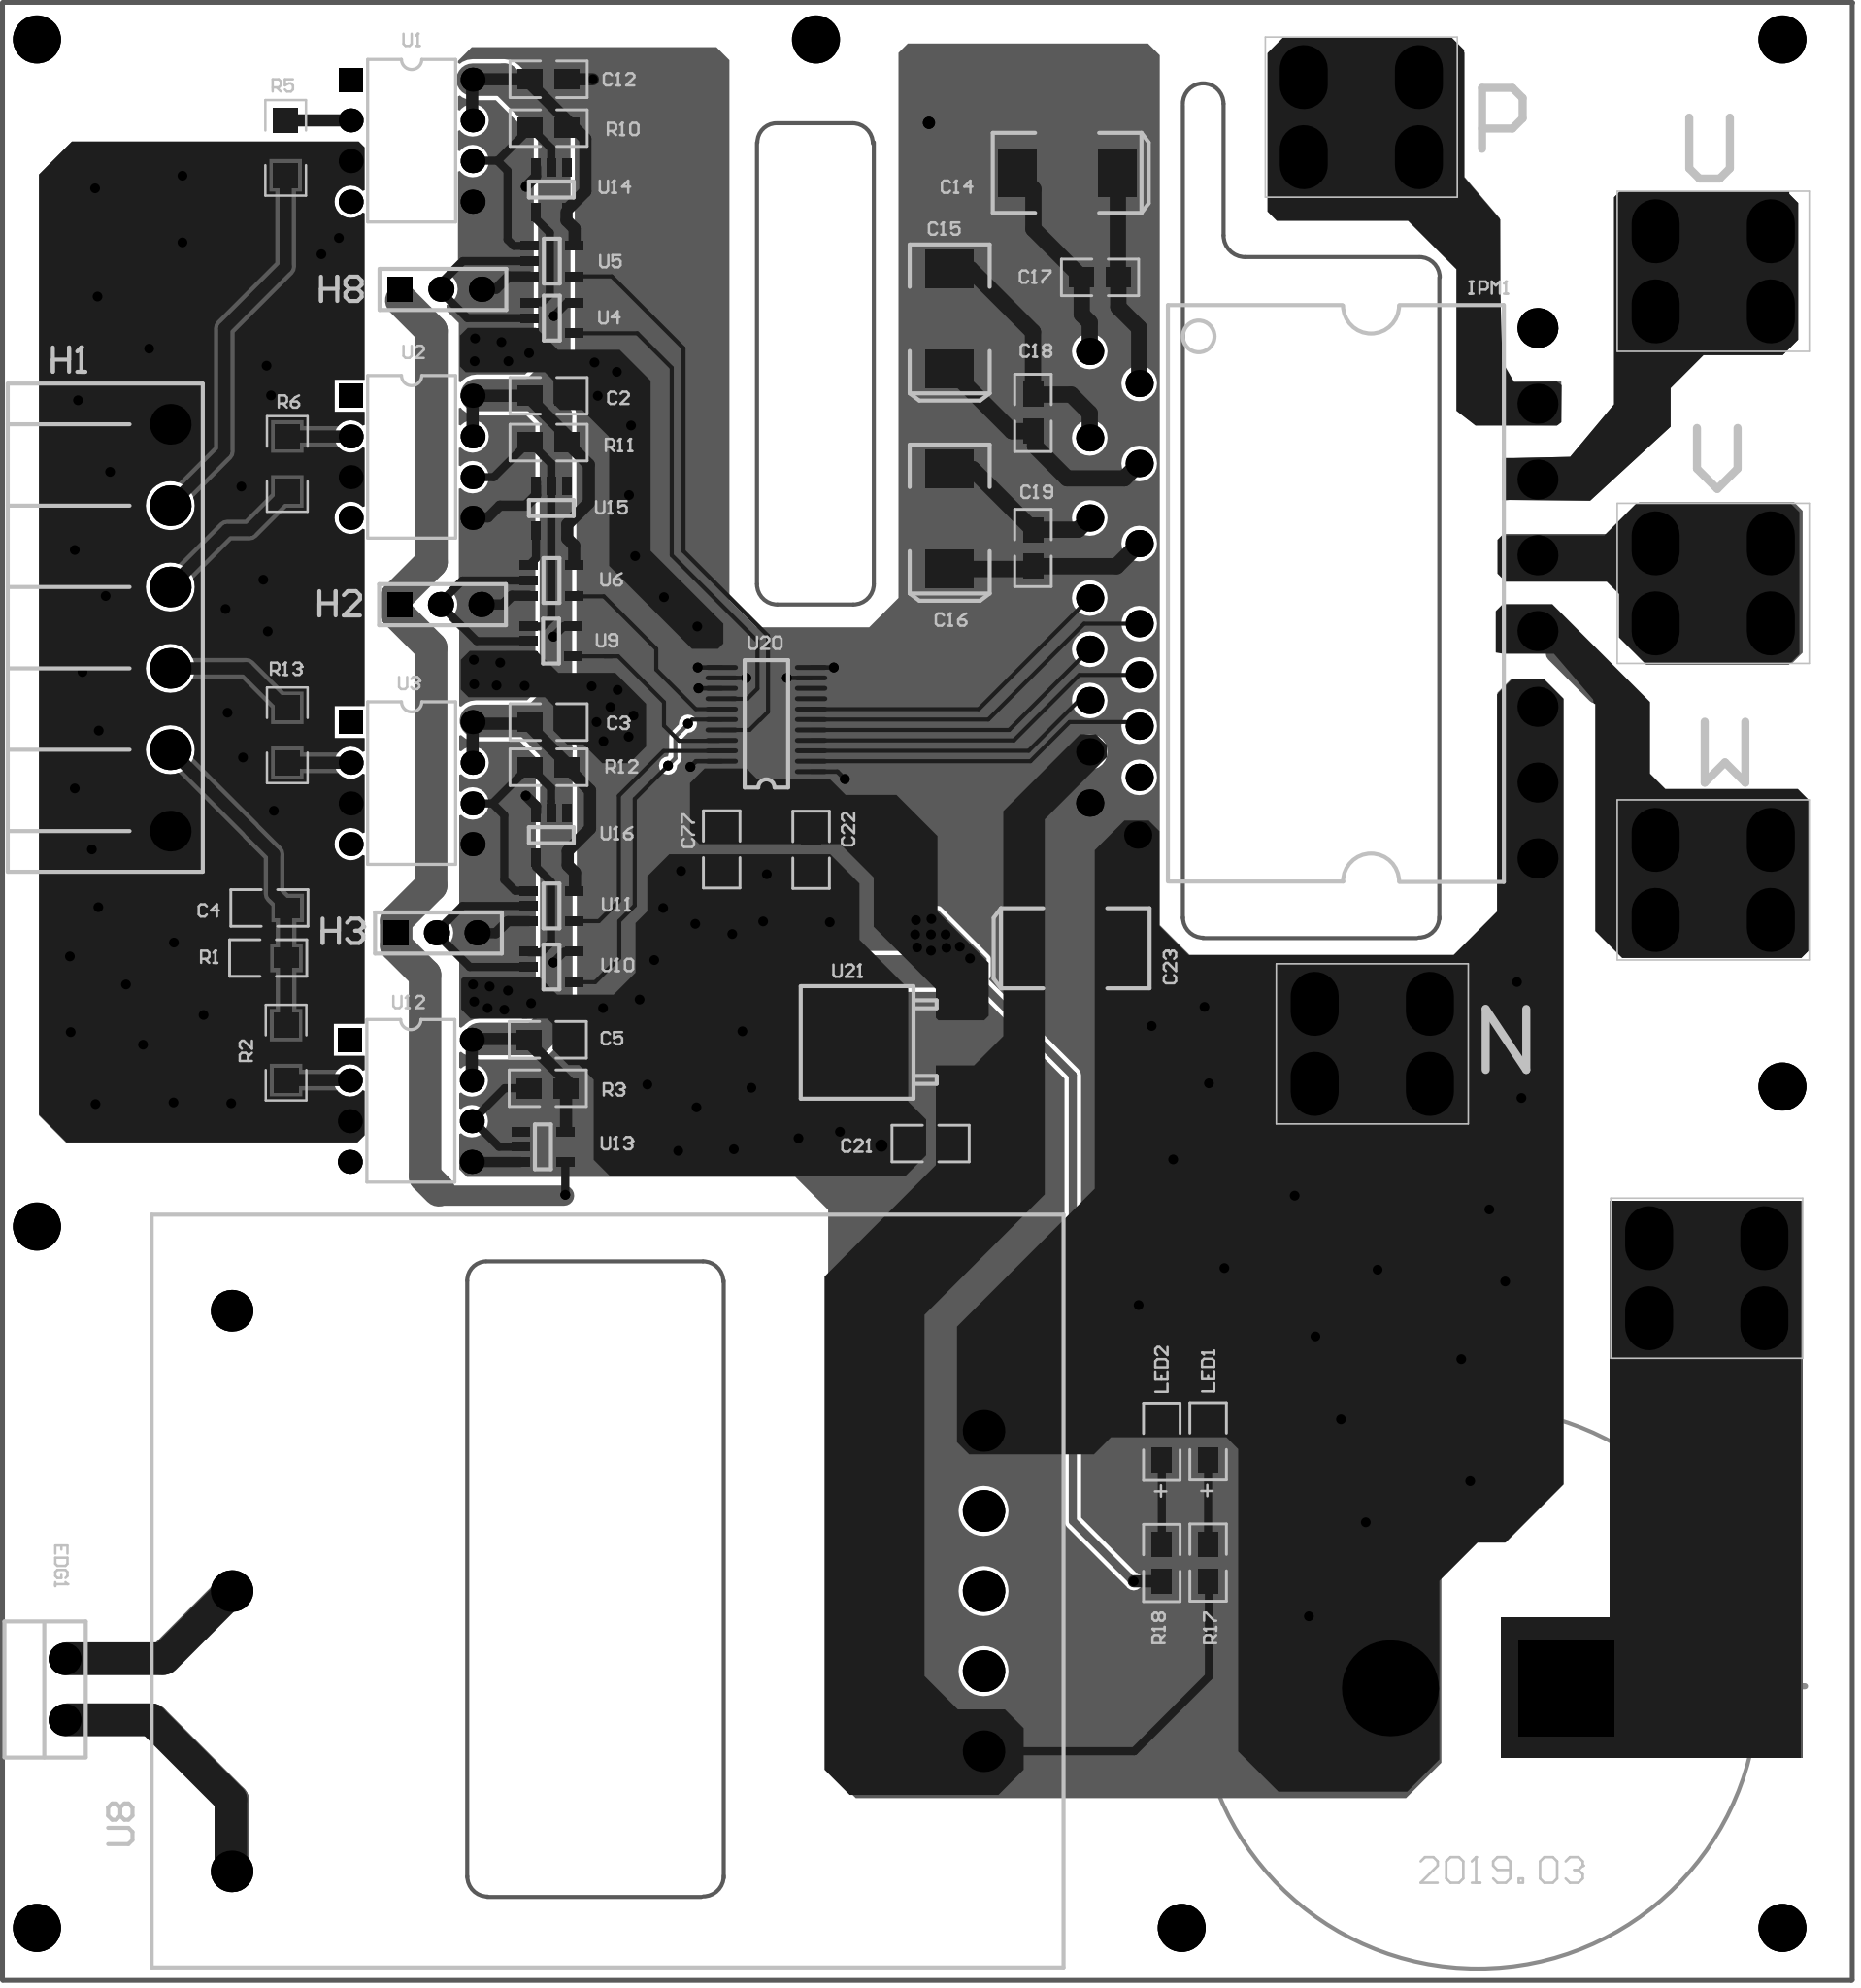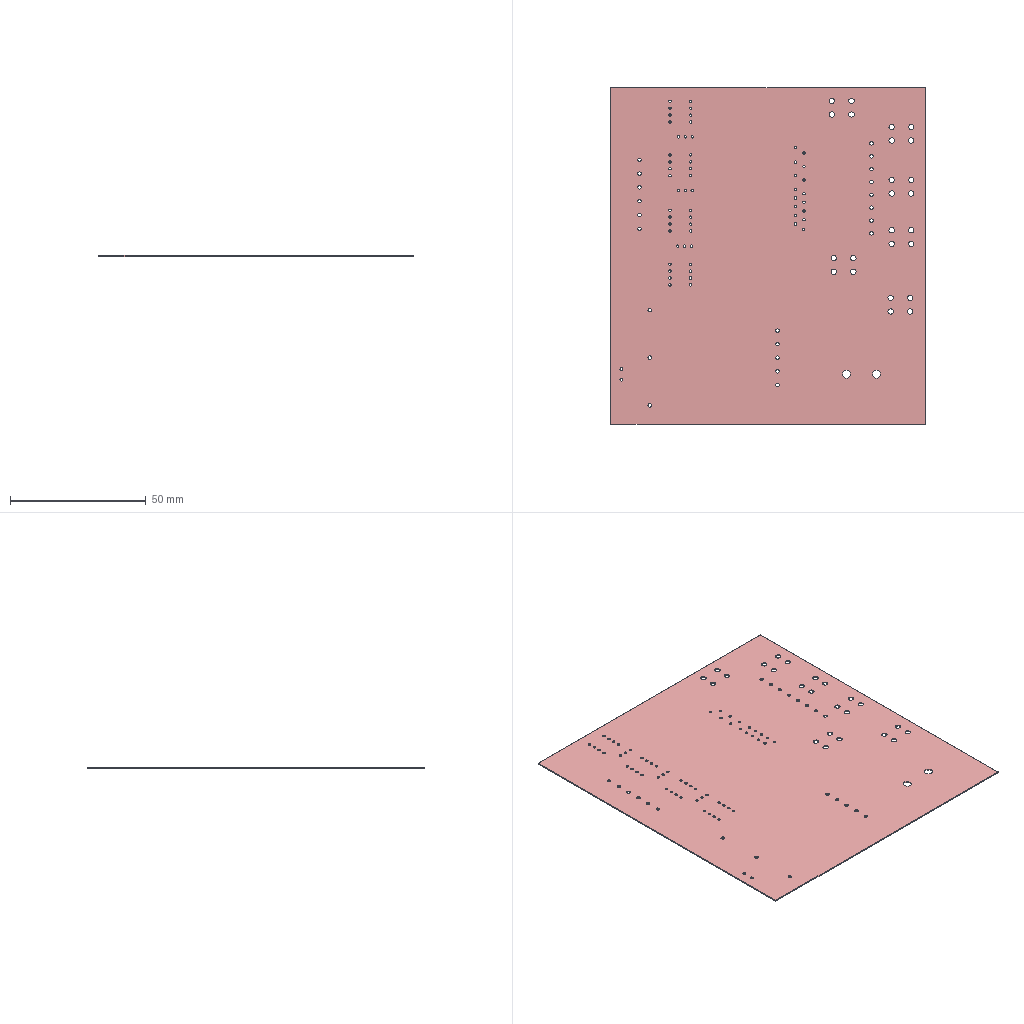Circuit board layout | Altium Designer | box 115.9 x 123.7 x 0.4 mm
Layer stack:
# Altium Designer layer stack of  (unit mm; dielectric type: 0 none, 1 core, 2 prepreg, 3 surface material)
index,name,kind,layer,copper_thickness_mm,dielectric_type,dielectric_thickness_mm,dielectric_material,dielectric_constant
0,Top Paste,other,,,,,,
1,Top Overlay,other,,,,,,
2,Top Solder,dielectric,,,3,0.0102,Solder Resist,3.5
3,Top Layer,copper,Top Layer,0.0356,,,,
4,Dielectric1,dielectric,,,0,0.32,FR-4,4.8
5,Bottom Layer,copper,Bottom Layer,0.0356,,,,
6,Bottom Solder,dielectric,,,3,0.0102,Solder Resist,3.5
7,Bottom Overlay,other,,,,,,
8,Bottom Paste,other,,,,,,
# drill layer pairs: low layer,high layer
drill_pair,Top Layer,Bottom Layer
Part placement:
Designator,Comment,Layer,Footprint,Center-X(mm),Center-Y(mm),Rotation
C22,0.01uF,TopLayer,0805,50.495,70.485,90
C1,450V,BottomLayer,ElecCap_450V,92.177,18.136,180
C19,0.1uF,TopLayer,0805,64.364,89.332,90
C15,22uF/35V,TopLayer,7343_CASE-D,59.157,103.632,270
C18,0.1uF,TopLayer,0805,64.364,97.765,90
C14,22uF/35V,TopLayer,7343_CASE-D,66.497,112.751,360
C16,22uF/35V,TopLayer,7343_CASE-D,59.157,91.135,270
C23,22uF/35V,TopLayer,7343_CASE-D,67.005,64.338,180
C17,0.1uF,TopLayer,0805,68.555,106.223,180
U21,L78M05,TopLayer,TO-252-2(DPAK),56.696,58.471,360
U20,SN74LVC8T245,TopLayer,SN74LVC8T245_TSSOP24,47.701,78.293,180
R13,500R,TopLayer,1206,17.755,77.635,90
R5,500R,TopLayer,1206,17.653,114.313,270
R6,500R,TopLayer,1206,17.755,94.577,270
U6,SN74AHC1G08,TopLayer,SOT-23-5,34.265,87.3,180
U5,SN74AHC1G08,TopLayer,SOT-23-5,34.29,107.239,180
U4,SN74AHC1G08,TopLayer,SOT-23-5,34.29,103.683,180
U3,6N137,TopLayer,DIP-8,25.527,74.651,360
U1,6N137,TopLayer,DIP-8,25.527,114.757,360
W1,PCBTerminator,TopLayer,PCBTerminator,106.883,68.605,90
IPM1,IKCM15F60GA,TopLayer,IKCM15F60GA,81.904,86.509,90
EDG1,EDG 2p,TopLayer,EDGCon_2p_3.81mm,3.835,18.059,270
N1,PCBTerminator,TopLayer,PCBTerminator,85.573,58.369,90
P1,PCBTerminator,TopLayer,PCBTerminator,84.887,116.23,90
U7,PCBTerminator,TopLayer,PCBTerminator,106.883,106.604,90
V1,PCBTerminator,TopLayer,PCBTerminator,106.883,87.122,90
C21,0.33uF,TopLayer,0805,57.963,52.146,360
U2,6N137,TopLayer,DIP-8,25.527,95.021,360
R10,10k,TopLayer,0805,34.087,115.545,360
H8,Header3,TopLayer,PinHeader3_2.54mm,27.356,105.486,360
LED1,LED,TopLayer,0805_LED,75.311,33.553,90
LED2,LED,TopLayer,0805_LED,72.415,33.528,90
R17,10k,TopLayer,0805,75.311,25.984,270
R18,3.3k,TopLayer,0805,72.415,25.959,270
U8,YAS5-15-W,TopLayer,YAS5,37.775,24.207,180
C77,0.1uF,TopLayer,0805,44.907,70.51,270
P2,PCBTerminator,TopLayer,PCBTerminator,106.477,43.739,90
U9,SN74AHC1G08,TopLayer,SOT-23-5,34.239,83.515,180
U10,SN74AHC1G08,TopLayer,SOT-23-5,34.265,63.17,180
U11,SN74AHC1G08,TopLayer,SOT-23-5,34.265,66.98,180
H1,Header6,TopLayer,EDGCon_6P_5.08mm,10.439,84.353,270
C4,30pF,TopLayer,0805,16.637,66.853,360
C5,0.1uF,TopLayer,0805,34.036,58.623,180
H2,Header3,TopLayer,PinHeader3_2.54mm,27.33,85.801,360
H3,Header3,TopLayer,PinHeader3_2.54mm,27.076,65.303,360
R1,10k,TopLayer,0805,16.561,63.729,360
R2,500R,TopLayer,1206,17.678,57.823,90
R3,10k,TopLayer,0805,34.036,55.601,360
U12,6N137,TopLayer,DIP-8,25.476,54.813,360
U13,SN74AHC1G04,TopLayer,SOT-23-5,33.731,51.943,180
C2,0.1uF,TopLayer,0805,34.087,98.831,180
C3,0.1uF,TopLayer,0805,34.087,78.461,180
C12,0.1uF,TopLayer,0805,34.087,118.593,180
R11,10k,TopLayer,0805,34.087,95.91,360
R12,10k,TopLayer,0805,34.087,75.641,360
U14,SN74AHC1G04,TopLayer,SOT-23-5,34.256,111.709,90
U15,SN74AHC1G04,TopLayer,SOT-23-5,34.256,91.821,90
U16,SN74AHC1G04,TopLayer,SOT-23-5,34.256,71.399,90
Pad and via stacks:
# Altium Designer via and pad stacks of  (unit mm). Each distinct definition once, with the count of objects using it.
# via: kind,start_layer,end_layer,hole_mm,diameter_mm,mode(0 simple;1 top-mid-bottom;2 full stack),diameter_per_layer,count,example_net
# pad: kind,layer,hole_mm,hole_type(0 round;1 square;2 slot),plating,top_size,top_shape(1 round;2 rect;3 octagon;9 rounded rect),mid_size,bottom_size,mode,footprint,size_per_layer,count,example
pad,Top Layer,0,0,plated,2.4x3,2,2.4x3,2.4x3,0,7343_CASE-D,,8,C23.1
pad,Top Layer,0,0,plated,1.524x1.27,2,1.524x1.27,1.524x1.27,0,0805,,36,C19.2
pad,Top Layer,0,0,plated,1.524x1.27,2,1.524x1.27,1.524x1.27,0,0805_LED,,4,LED2.K
pad,Top Layer,0,0,plated,1.524x1.524,2,1.524x1.524,1.524x1.524,0,1206,,8,R6.2
pad,Top Layer,0,0,plated,1.5x2.8,2,1.5x2.8,1.5x2.8,0,TO-252-2(DPAK),,2,U21.2
pad,Top Layer,0,0,plated,6.3x6.3,2,6.3x6.3,6.3x6.3,0,TO-252-2(DPAK),,1,U21.1
pad,Top Layer,0,0,plated,2.032x0.3048,1,2.032x0.3048,2.032x0.3048,0,SN74LVC8T245_TSSOP24,,23,U20.14
pad,Top Layer,0,0,plated,2.032x0.3048,2,2.032x0.3048,2.032x0.3048,0,SN74LVC8T245_TSSOP24,,1,U20.1
pad,Top Layer,0,0,plated,0.6x1.1,2,0.6x1.1,0.6x1.1,0,SOT-23-5,,50,U11.1
pad,Multi-Layer,0.8636,0,plated,1.575x1.575,1,1.575x1.575,1.575x1.575,0,PinHeader3_2.54mm,,6,H8.2
pad,Multi-Layer,0.8636,0,plated,1.575x1.575,2,1.575x1.575,1.575x1.575,0,PinHeader3_2.54mm,,3,H8.1
pad,Multi-Layer,0.9,0,plated,1.5x1.5,1,1.5x1.5,1.5x1.5,0,DIP-8,,28,U2.5
pad,Multi-Layer,0.9,0,plated,1.5x1.5,2,1.5x1.5,1.5x1.5,0,DIP-8,,4,U2.1
pad,Multi-Layer,1.1,0,plated,2x2,1,2x2,2x2,0,EDGCon_2p_3.81mm,,2,EDG1.1
pad,Multi-Layer,0.9,0,plated,1.7x1.7,1,1.7x1.7,1.7x1.7,0,IKCM15F60GA,,16,IPM1.4
pad,Multi-Layer,1.3,0,plated,2.5x2.5,1,2.5x2.5,2.5x2.5,0,IKCM15F60GA,,8,IPM1.24
pad,Multi-Layer,2,0,plated,4x3,1,4x3,4x3,0,PCBTerminator,,24,W1.1
pad,Multi-Layer,1.321,0,plated,2.6x2.6,1,2.6x2.6,2.6x2.6,0,YAS5,,8,U8.8
pad,Multi-Layer,3,0,plated,6x6,2,6x6,6x6,0,ElecCap_450V,,1,C1.1
pad,Multi-Layer,3,0,plated,6x6,1,6x6,6x6,0,ElecCap_450V,,1,C1.2
pad,Multi-Layer,1.295,0,plated,2.54x2.54,1,2.54x2.54,2.54x2.54,0,EDGCon_6P_5.08mm,,6,H1.5
via,Top Layer,Bottom Layer,3,3,0,,8,
via,Top Layer,Bottom Layer,0.381,0.762,0,,2,IPM_N
via,Top Layer,Bottom Layer,0.3048,0.6096,0,,154,PWM_WH
Copper pours:
name,layer,net,type(0 solid;1 hatched;2 none)
Top Layer-No Net,Top Layer,+5V_IPM,0
Top Layer-No Net,Top Layer,GND,0
Top Layer-No Net,Top Layer,IPM_N,0
Top Layer-No Net,Top Layer,IPM_N,0
Top Layer-No Net,Top Layer,IPM_N,0
Top Layer-No Net,Top Layer,IPM_N,0
Top Layer-No Net,Top Layer,IPM_N,0
Top Layer-No Net,Bottom Layer,+5V_IPM,0
Top Layer-No Net,Bottom Layer,GND,0
Top Layer-No Net,Bottom Layer,IPM_N,0
Design rules, without the lines most boards share:
# Altium Designer design rules of  (exported by Altium Designer, unit mm)
# columns: name | kind | enabled | priority | scope1 | scope2 | descriptor | typed fields (field=value)
Clearance | 0 | enabled | 1 | All | All | Clearance Constraint (Gap=10mil) (All),(All) | gap=0.254
PlaneConnect | 6 | enabled | 1 | All | All | Power Plane Connect Rule(Direct Connect )(Expansion=20mil) (Conductor Width=10mil) (Air Gap=10mil) (Entries=4) (All) | relief_conductor_width=0.254 relief_entries=4 relief_expansion=0.508
PolygonConnect | 20 | enabled | 1 | All | All | Polygon Connect Rule(Direct Connect )(Conductor Width=75mil) (Relief Angle=90 Angle) (Entries=4) (Air Gap Width=10mil) (All),(All) | connect_style(0=relief,1=direct,2=none)=1 relief_conductor_width=1.905 relief_entries=4
Width | 2 | enabled | 1 | All | All | Width Constraint (Min=10mil) (Max=99mil) (Preferred=11.811mil) (All) |
RoutingVias | 11 | enabled | 1 | All | All | Routing Via (MinHoleWidth=12mil) (MaxHoleWidth=12mil) (PreferredHoleWidth=12mil) (MinWidth=24mil) (MaxWidth=24mil) (PreferedWidth=24mil) (All) | via_min_hole=0.3048 via_max_hole=0.3048 via_preferred_diameter=0.6096 via_preferred_hole=0.3048
PasteMaskExpansion | 14 | enabled | 1 | All | All | Paste Mask Expansion (Expansion =0mil) (All) | expansion=0
SolderMaskExpansion | 13 | enabled | 1 | All | All | Solder Mask Expansion (Expansion =4mil) (All) | expansion=0.1016
TestPointUsage | 44 | enabled | 1 | All | All | Fabrication Testpoint Usage (Valid =One Required, Allow multiple per net=No) (All) |
Testpoint | 43 | enabled | 1 | (IsPad And (OnTopLayer Or OnBottomLayer)) | All | Fabrication Testpoint Style (Under Component=Yes) ((IsPad And (OnTopLayer Or OnBottomLayer))) |
ComponentClearance | 24 | disabled | 1 | All | All | Component Clearance Constraint ( Horizontal Gap = 10mil, Vertical Gap = 10mil ) (Disabled)(All),(All)  | gap=0.254
Height | 50 | disabled | 1 | All | All | Height Constraint (Min=0mil) (Max=1000mil) (Prefered=500mil) (Disabled)(All) | min_height=0 max_height=25.4
HoleSize | 42 | enabled | 1 | All | All | Hole Size Constraint (Min=6mil) (Max=150mil) (All) |
Fanout_Default | 49 | enabled | 4 | All | All | Fanout Control Rule ( (All) ) |
Fanout_Small | 49 | disabled | 5 | All | All | Fanout Control Rule ( (Disabled)(All) ) |
Fanout_SOIC | 49 | disabled | 3 | All | All | Fanout Control Rule ( (Disabled)(All) ) |
Fanout_LCC | 49 | disabled | 1 | All | All | Fanout Control Rule ( (Disabled)(All) ) |
Fanout_BGA | 49 | disabled | 2 | All | All | Fanout Control Rule ( (Disabled)(All) ) |
DiffPairsRouting | 51 | enabled | 1 | All | All | Differential Pairs Uncoupled Length using the Gap Constraints (Min=10mil) (Max=10mil) (Prefered=10mil)  and Width Constraints (Min=15mil) (Max=15mil) (Prefered=15mil) (All) |
HoleToHoleClearance | 52 | enabled | 1 | All | All | Hole To Hole Clearance (Gap=10mil) (All),(All) | gap=0.254
MinimumSolderMaskSliver | 53 | enabled | 1 | All | All | Minimum Solder Mask Sliver (Gap=0mil) (All),(All) |
SilkscreenOverComponentPads | 54 | disabled | 1 | IsPad | All | Silk To Solder Mask (Clearance=10mil) (Disabled)(IsPad),(All) |
SilkToSilkClearance | 55 | enabled | 1 | All | All | Silk to Silk (Clearance=0mil) (All),(All) |